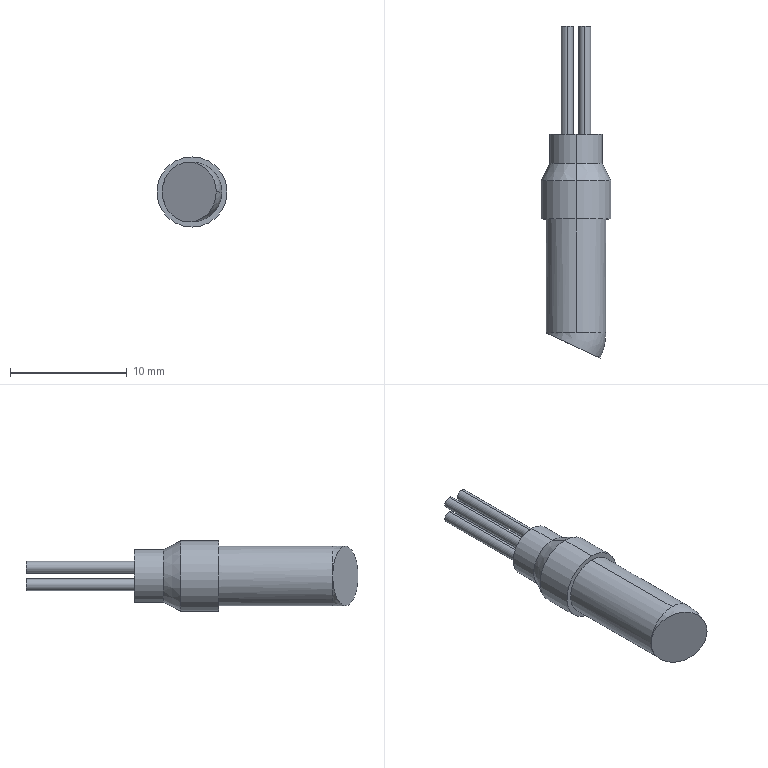Part | SolidWorks | features BaseBody 1 | 1 solid | 25 faces | box 6 x 28.381 x 6 mm | volume 414.888 mm3 | cylinder 14 | plane 7 | spline 2 | cone 2 | commonest cylinder face diameters 1 x8 4.5 x2 5.1 x2 6 x2
STEP:
#1=CARTESIAN_POINT('',(2.55,68.684,0.));
#2=VERTEX_POINT('',#1);
#3=CARTESIAN_POINT('',(0.,68.684,-2.55));
#4=VERTEX_POINT('',#3);
#5=CARTESIAN_POINT('',(0.,68.684,0.));
#6=DIRECTION('',(0.,1.,0.));
#7=DIRECTION('',(0.,0.,1.));
#8=AXIS2_PLACEMENT_3D('',#5,#6,#7);
#9=CIRCLE('',#8,2.55);
#10=EDGE_CURVE('',#2,#4,#9,.T.);
#11=ORIENTED_EDGE('',*,*,#10,.T.);
#12=CARTESIAN_POINT('',(0.,78.399,-2.55));
#13=VERTEX_POINT('',#12);
#14=CARTESIAN_POINT('',(0.,80.649,-2.55));
#15=DIRECTION('',(0.,1.,0.));
#16=VECTOR('',#15,1000.);
#17=LINE('',#14,#16);
#18=EDGE_CURVE('',#4,#13,#17,.T.);
#19=ORIENTED_EDGE('',*,*,#18,.T.);
#20=CARTESIAN_POINT('',(0.,78.399,2.55));
#21=VERTEX_POINT('',#20);
#22=CARTESIAN_POINT('',(0.,78.399,0.));
#23=DIRECTION('',(0.,-1.,0.));
#24=DIRECTION('',(0.,0.,1.));
#25=AXIS2_PLACEMENT_3D('',#22,#23,#24);
#26=CIRCLE('',#25,2.55);
#27=EDGE_CURVE('',#13,#21,#26,.T.);
#28=ORIENTED_EDGE('',*,*,#27,.T.);
#29=CARTESIAN_POINT('',(0.,68.684,2.55));
#30=VERTEX_POINT('',#29);
#31=CARTESIAN_POINT('',(0.,80.649,2.55));
#32=DIRECTION('',(0.,1.,0.));
#33=VECTOR('',#32,1000.);
#34=LINE('',#31,#33);
#35=EDGE_CURVE('',#30,#21,#34,.T.);
#36=ORIENTED_EDGE('',*,*,#35,.F.);
#37=CARTESIAN_POINT('',(0.,68.684,0.));
#38=DIRECTION('',(0.,1.,0.));
#39=DIRECTION('',(0.,0.,1.));
#40=AXIS2_PLACEMENT_3D('',#37,#38,#39);
#41=CIRCLE('',#40,2.55);
#42=EDGE_CURVE('',#30,#2,#41,.T.);
#43=ORIENTED_EDGE('',*,*,#42,.T.);
#44=EDGE_LOOP('',(#11,#19,#28,#36,#43));
#45=FACE_OUTER_BOUND('',#44,.T.);
#46=CARTESIAN_POINT('',(0.,80.649,0.));
#47=DIRECTION('',(0.,1.,0.));
#48=DIRECTION('',(0.,0.,1.));
#49=AXIS2_PLACEMENT_3D('',#46,#47,#48);
#50=CYLINDRICAL_SURFACE('',#49,2.55);
#51=ADVANCED_FACE('',(#45),#50,.T.);
#52=CARTESIAN_POINT('',(2.069,66.514,0.));
#53=VERTEX_POINT('',#52);
#54=CARTESIAN_POINT('',(-2.553,68.67,0.));
#55=VERTEX_POINT('',#54);
#56=CARTESIAN_POINT('',(2.069,66.514,0.));
#57=CARTESIAN_POINT('',(2.069,66.514,-0.1685));
#58=CARTESIAN_POINT('',(2.054,66.521,-0.3342));
#59=CARTESIAN_POINT('',(1.995,66.549,-0.6601));
#60=CARTESIAN_POINT('',(1.951,66.569,-0.822));
#61=CARTESIAN_POINT('',(1.835,66.623,-1.131));
#62=CARTESIAN_POINT('',(1.764,66.657,-1.277));
#63=CARTESIAN_POINT('',(1.596,66.735,-1.555));
#64=CARTESIAN_POINT('',(1.498,66.78,-1.686));
#65=CARTESIAN_POINT('',(1.285,66.88,-1.921));
#66=CARTESIAN_POINT('',(1.169,66.934,-2.027));
#67=CARTESIAN_POINT('',(0.916,67.052,-2.213));
#68=CARTESIAN_POINT('',(0.7815,67.115,-2.292));
#69=CARTESIAN_POINT('',(0.5033,67.244,-2.419));
#70=CARTESIAN_POINT('',(0.3577,67.312,-2.468));
#71=CARTESIAN_POINT('',(0.05933,67.451,-2.534));
#72=CARTESIAN_POINT('',(-0.09064,67.521,-2.55));
#73=CARTESIAN_POINT('',(-0.3921,67.662,-2.55));
#74=CARTESIAN_POINT('',(-0.5452,67.733,-2.533));
#75=CARTESIAN_POINT('',(-0.8416,67.871,-2.468));
#76=CARTESIAN_POINT('',(-0.9857,67.939,-2.42));
#77=CARTESIAN_POINT('',(-1.266,68.069,-2.292));
#78=CARTESIAN_POINT('',(-1.401,68.132,-2.213));
#79=CARTESIAN_POINT('',(-1.651,68.249,-2.028));
#80=CARTESIAN_POINT('',(-1.768,68.303,-1.923));
#81=CARTESIAN_POINT('',(-1.984,68.404,-1.685));
#82=CARTESIAN_POINT('',(-2.08,68.449,-1.555));
#83=CARTESIAN_POINT('',(-2.247,68.527,-1.279));
#84=CARTESIAN_POINT('',(-2.319,68.561,-1.13));
#85=CARTESIAN_POINT('',(-2.435,68.615,-0.8212));
#86=CARTESIAN_POINT('',(-2.479,68.635,-0.6622));
#87=CARTESIAN_POINT('',(-2.538,68.663,-0.3354));
#88=CARTESIAN_POINT('',(-2.553,68.67,-0.1664));
#89=CARTESIAN_POINT('',(-2.553,68.67,0.));
#90=B_SPLINE_CURVE_WITH_KNOTS('',3,(#56,#57,#58,#59,#60,#61,#62,#63,#64,#65,#66,#67,#68,#69,#70,#71,#72,#73,#74,#75,#76,#77,#78,#79,#80,#81,#82,#83,#84,#85,#86,#87,#88,#89),.UNSPECIFIED.,.F.,.F.,(4,2,2,2,2,2,2,2,2,2,2,2,2,2,2,2,4),(0.,0.0004983,0.0009966,0.001495,0.001993,0.002491,0.00299,0.003488,0.003986,0.004485,0.004983,0.005481,0.005979,0.006478,0.006976,0.007474,0.007972),.UNSPECIFIED.);
#91=EDGE_CURVE('',#53,#55,#90,.T.);
#92=ORIENTED_EDGE('',*,*,#91,.T.);
#93=CARTESIAN_POINT('',(-2.55,68.684,0.));
#94=VERTEX_POINT('',#93);
#95=CARTESIAN_POINT('',(-2.585,68.684,0.));
#96=DIRECTION('',(0.,0.,1.));
#97=DIRECTION('',(1.,0.,0.));
#98=AXIS2_PLACEMENT_3D('',#95,#96,#97);
#99=CIRCLE('',#98,0.035);
#100=EDGE_CURVE('',#55,#94,#99,.T.);
#101=ORIENTED_EDGE('',*,*,#100,.T.);
#102=CARTESIAN_POINT('',(0.,68.684,0.));
#103=DIRECTION('',(0.,1.,0.));
#104=DIRECTION('',(0.,0.,1.));
#105=AXIS2_PLACEMENT_3D('',#102,#103,#104);
#106=CIRCLE('',#105,2.55);
#107=EDGE_CURVE('',#4,#94,#106,.T.);
#108=ORIENTED_EDGE('',*,*,#107,.F.);
#109=ORIENTED_EDGE('',*,*,#10,.F.);
#110=CARTESIAN_POINT('',(-2.585,68.684,0.));
#111=DIRECTION('',(0.,0.,1.));
#112=DIRECTION('',(1.,0.,0.));
#113=AXIS2_PLACEMENT_3D('',#110,#111,#112);
#114=CIRCLE('',#113,5.135);
#115=EDGE_CURVE('',#53,#2,#114,.T.);
#116=ORIENTED_EDGE('',*,*,#115,.F.);
#117=EDGE_LOOP('',(#92,#101,#108,#109,#116));
#118=FACE_OUTER_BOUND('',#117,.T.);
#119=CARTESIAN_POINT('',(2.069,66.514,0.));
#120=CARTESIAN_POINT('',(2.387,67.197,0.));
#121=CARTESIAN_POINT('',(2.55,67.932,0.));
#122=CARTESIAN_POINT('',(2.55,68.684,0.));
#123=CARTESIAN_POINT('',(2.069,66.514,-5.1));
#124=CARTESIAN_POINT('',(2.387,67.197,-5.1));
#125=CARTESIAN_POINT('',(2.55,67.932,-5.1));
#126=CARTESIAN_POINT('',(2.55,68.684,-5.1));
#127=CARTESIAN_POINT('',(-2.553,68.67,-5.1));
#128=CARTESIAN_POINT('',(-2.551,68.674,-5.1));
#129=CARTESIAN_POINT('',(-2.55,68.679,-5.1));
#130=CARTESIAN_POINT('',(-2.55,68.684,-5.1));
#131=CARTESIAN_POINT('',(-2.553,68.67,0.));
#132=CARTESIAN_POINT('',(-2.551,68.674,0.));
#133=CARTESIAN_POINT('',(-2.55,68.679,0.));
#134=CARTESIAN_POINT('',(-2.55,68.684,0.));
#135=(BOUNDED_SURFACE()B_SPLINE_SURFACE(3,3,((#119,#120,#121,#122),(#123,#124,#125,#126),(#127,#128,#129,#130),(#131,#132,#133,#134)),.UNSPECIFIED.,.F.,.F.,.F.)B_SPLINE_SURFACE_WITH_KNOTS((4,4),(4,4),(0.,1.),(0.,1.),.UNSPECIFIED.)GEOMETRIC_REPRESENTATION_ITEM()RATIONAL_B_SPLINE_SURFACE(((1.,0.9842,0.9842,1.),(0.3333,0.3281,0.3281,0.3333),(0.3333,0.3281,0.3281,0.3333),(1.,0.9842,0.9842,1.)))REPRESENTATION_ITEM('')SURFACE());
#136=ADVANCED_FACE('',(#118),#135,.T.);
#137=CARTESIAN_POINT('',(0.,78.399,3.));
#138=VERTEX_POINT('',#137);
#139=CARTESIAN_POINT('',(0.,78.399,-3.));
#140=VERTEX_POINT('',#139);
#141=CARTESIAN_POINT('',(0.,78.399,0.));
#142=DIRECTION('',(0.,1.,0.));
#143=DIRECTION('',(0.,0.,1.));
#144=AXIS2_PLACEMENT_3D('',#141,#142,#143);
#145=CIRCLE('',#144,3.);
#146=EDGE_CURVE('',#138,#140,#145,.T.);
#147=ORIENTED_EDGE('',*,*,#146,.T.);
#148=CARTESIAN_POINT('',(0.,81.649,-3.));
#149=VERTEX_POINT('',#148);
#150=CARTESIAN_POINT('',(0.,78.399,-3.));
#151=DIRECTION('',(0.,1.,0.));
#152=VECTOR('',#151,1000.);
#153=LINE('',#150,#152);
#154=EDGE_CURVE('',#140,#149,#153,.T.);
#155=ORIENTED_EDGE('',*,*,#154,.T.);
#156=CARTESIAN_POINT('',(0.,81.649,3.));
#157=VERTEX_POINT('',#156);
#158=CARTESIAN_POINT('',(0.,81.649,0.));
#159=DIRECTION('',(0.,-1.,0.));
#160=DIRECTION('',(0.,0.,1.));
#161=AXIS2_PLACEMENT_3D('',#158,#159,#160);
#162=CIRCLE('',#161,3.);
#163=EDGE_CURVE('',#149,#157,#162,.T.);
#164=ORIENTED_EDGE('',*,*,#163,.T.);
#165=CARTESIAN_POINT('',(0.,78.399,3.));
#166=DIRECTION('',(0.,1.,0.));
#167=VECTOR('',#166,1000.);
#168=LINE('',#165,#167);
#169=EDGE_CURVE('',#138,#157,#168,.T.);
#170=ORIENTED_EDGE('',*,*,#169,.F.);
#171=EDGE_LOOP('',(#147,#155,#164,#170));
#172=FACE_OUTER_BOUND('',#171,.T.);
#173=CARTESIAN_POINT('',(0.,78.399,0.));
#174=DIRECTION('',(0.,1.,0.));
#175=DIRECTION('',(0.,0.,1.));
#176=AXIS2_PLACEMENT_3D('',#173,#174,#175);
#177=CYLINDRICAL_SURFACE('',#176,3.);
#178=ADVANCED_FACE('',(#172),#177,.T.);
#179=CARTESIAN_POINT('',(0.,83.149,-2.25));
#180=VERTEX_POINT('',#179);
#181=CARTESIAN_POINT('',(0.,83.149,2.25));
#182=VERTEX_POINT('',#181);
#183=CARTESIAN_POINT('',(0.,83.149,0.));
#184=DIRECTION('',(0.,-1.,0.));
#185=DIRECTION('',(0.,0.,-1.));
#186=AXIS2_PLACEMENT_3D('',#183,#184,#185);
#187=CIRCLE('',#186,2.25);
#188=EDGE_CURVE('',#180,#182,#187,.T.);
#189=ORIENTED_EDGE('',*,*,#188,.T.);
#190=CARTESIAN_POINT('',(0.,81.649,3.));
#191=DIRECTION('',(0.,-0.8944,0.4472));
#192=VECTOR('',#191,1000.);
#193=LINE('',#190,#192);
#194=EDGE_CURVE('',#182,#157,#193,.T.);
#195=ORIENTED_EDGE('',*,*,#194,.T.);
#196=ORIENTED_EDGE('',*,*,#163,.F.);
#197=CARTESIAN_POINT('',(0.,81.649,-3.));
#198=DIRECTION('',(0.,-0.8944,-0.4472));
#199=VECTOR('',#198,1000.);
#200=LINE('',#197,#199);
#201=EDGE_CURVE('',#180,#149,#200,.T.);
#202=ORIENTED_EDGE('',*,*,#201,.F.);
#203=EDGE_LOOP('',(#189,#195,#196,#202));
#204=FACE_OUTER_BOUND('',#203,.T.);
#205=CARTESIAN_POINT('',(0.,81.649,0.));
#206=DIRECTION('',(0.,-1.,0.));
#207=DIRECTION('',(0.,0.,-1.));
#208=AXIS2_PLACEMENT_3D('',#205,#206,#207);
#209=CONICAL_SURFACE('',#208,3.,0.4636);
#210=ADVANCED_FACE('',(#204),#209,.T.);
#211=ORIENTED_EDGE('',*,*,#188,.F.);
#212=CARTESIAN_POINT('',(0.,85.649,-2.25));
#213=VERTEX_POINT('',#212);
#214=CARTESIAN_POINT('',(0.,78.399,-2.25));
#215=DIRECTION('',(0.,1.,0.));
#216=VECTOR('',#215,1000.);
#217=LINE('',#214,#216);
#218=EDGE_CURVE('',#180,#213,#217,.T.);
#219=ORIENTED_EDGE('',*,*,#218,.T.);
#220=CARTESIAN_POINT('',(0.,85.649,2.25));
#221=VERTEX_POINT('',#220);
#222=CARTESIAN_POINT('',(0.,85.649,0.));
#223=DIRECTION('',(0.,-1.,0.));
#224=DIRECTION('',(0.,0.,1.));
#225=AXIS2_PLACEMENT_3D('',#222,#223,#224);
#226=CIRCLE('',#225,2.25);
#227=EDGE_CURVE('',#213,#221,#226,.T.);
#228=ORIENTED_EDGE('',*,*,#227,.T.);
#229=CARTESIAN_POINT('',(0.,78.399,2.25));
#230=DIRECTION('',(0.,1.,0.));
#231=VECTOR('',#230,1000.);
#232=LINE('',#229,#231);
#233=EDGE_CURVE('',#182,#221,#232,.T.);
#234=ORIENTED_EDGE('',*,*,#233,.F.);
#235=EDGE_LOOP('',(#211,#219,#228,#234));
#236=FACE_OUTER_BOUND('',#235,.T.);
#237=CARTESIAN_POINT('',(0.,78.399,0.));
#238=DIRECTION('',(0.,1.,0.));
#239=DIRECTION('',(0.,0.,1.));
#240=AXIS2_PLACEMENT_3D('',#237,#238,#239);
#241=CYLINDRICAL_SURFACE('',#240,2.25);
#242=ADVANCED_FACE('',(#236),#241,.T.);
#243=CARTESIAN_POINT('',(0.75,85.649,-0.25));
#244=VERTEX_POINT('',#243);
#245=CARTESIAN_POINT('',(0.75,85.649,-1.25));
#246=VERTEX_POINT('',#245);
#247=CARTESIAN_POINT('',(0.75,85.649,-0.75));
#248=DIRECTION('',(0.,1.,0.));
#249=DIRECTION('',(0.,0.,1.));
#250=AXIS2_PLACEMENT_3D('',#247,#248,#249);
#251=CIRCLE('',#250,0.5);
#252=EDGE_CURVE('',#244,#246,#251,.T.);
#253=ORIENTED_EDGE('',*,*,#252,.T.);
#254=CARTESIAN_POINT('',(0.75,94.895,-1.25));
#255=VERTEX_POINT('',#254);
#256=CARTESIAN_POINT('',(0.75,94.895,-1.25));
#257=DIRECTION('',(0.,1.,0.));
#258=VECTOR('',#257,1000.);
#259=LINE('',#256,#258);
#260=EDGE_CURVE('',#246,#255,#259,.T.);
#261=ORIENTED_EDGE('',*,*,#260,.T.);
#262=CARTESIAN_POINT('',(0.75,94.895,-0.25));
#263=VERTEX_POINT('',#262);
#264=CARTESIAN_POINT('',(0.75,94.895,-0.75));
#265=DIRECTION('',(0.,-1.,0.));
#266=DIRECTION('',(0.,0.,1.));
#267=AXIS2_PLACEMENT_3D('',#264,#265,#266);
#268=CIRCLE('',#267,0.5);
#269=EDGE_CURVE('',#255,#263,#268,.T.);
#270=ORIENTED_EDGE('',*,*,#269,.T.);
#271=CARTESIAN_POINT('',(0.75,94.895,-0.25));
#272=DIRECTION('',(0.,1.,0.));
#273=VECTOR('',#272,1000.);
#274=LINE('',#271,#273);
#275=EDGE_CURVE('',#244,#263,#274,.T.);
#276=ORIENTED_EDGE('',*,*,#275,.F.);
#277=EDGE_LOOP('',(#253,#261,#270,#276));
#278=FACE_OUTER_BOUND('',#277,.T.);
#279=CARTESIAN_POINT('',(0.75,94.895,-0.75));
#280=DIRECTION('',(0.,1.,0.));
#281=DIRECTION('',(0.,0.,1.));
#282=AXIS2_PLACEMENT_3D('',#279,#280,#281);
#283=CYLINDRICAL_SURFACE('',#282,0.5);
#284=ADVANCED_FACE('',(#278),#283,.T.);
#285=CARTESIAN_POINT('',(-0.75,85.649,-0.25));
#286=VERTEX_POINT('',#285);
#287=CARTESIAN_POINT('',(-0.75,85.649,-1.25));
#288=VERTEX_POINT('',#287);
#289=CARTESIAN_POINT('',(-0.75,85.649,-0.75));
#290=DIRECTION('',(0.,1.,0.));
#291=DIRECTION('',(0.,0.,1.));
#292=AXIS2_PLACEMENT_3D('',#289,#290,#291);
#293=CIRCLE('',#292,0.5);
#294=EDGE_CURVE('',#286,#288,#293,.T.);
#295=ORIENTED_EDGE('',*,*,#294,.T.);
#296=CARTESIAN_POINT('',(-0.75,94.895,-1.25));
#297=VERTEX_POINT('',#296);
#298=CARTESIAN_POINT('',(-0.75,94.895,-1.25));
#299=DIRECTION('',(0.,1.,0.));
#300=VECTOR('',#299,1000.);
#301=LINE('',#298,#300);
#302=EDGE_CURVE('',#288,#297,#301,.T.);
#303=ORIENTED_EDGE('',*,*,#302,.T.);
#304=CARTESIAN_POINT('',(-0.75,94.895,-0.25));
#305=VERTEX_POINT('',#304);
#306=CARTESIAN_POINT('',(-0.75,94.895,-0.75));
#307=DIRECTION('',(0.,-1.,0.));
#308=DIRECTION('',(0.,0.,1.));
#309=AXIS2_PLACEMENT_3D('',#306,#307,#308);
#310=CIRCLE('',#309,0.5);
#311=EDGE_CURVE('',#297,#305,#310,.T.);
#312=ORIENTED_EDGE('',*,*,#311,.T.);
#313=CARTESIAN_POINT('',(-0.75,94.895,-0.25));
#314=DIRECTION('',(0.,1.,0.));
#315=VECTOR('',#314,1000.);
#316=LINE('',#313,#315);
#317=EDGE_CURVE('',#286,#305,#316,.T.);
#318=ORIENTED_EDGE('',*,*,#317,.F.);
#319=EDGE_LOOP('',(#295,#303,#312,#318));
#320=FACE_OUTER_BOUND('',#319,.T.);
#321=CARTESIAN_POINT('',(-0.75,94.895,-0.75));
#322=DIRECTION('',(0.,1.,0.));
#323=DIRECTION('',(0.,0.,1.));
#324=AXIS2_PLACEMENT_3D('',#321,#322,#323);
#325=CYLINDRICAL_SURFACE('',#324,0.5);
#326=ADVANCED_FACE('',(#320),#325,.T.);
#327=CARTESIAN_POINT('',(-0.75,85.649,1.25));
#328=VERTEX_POINT('',#327);
#329=CARTESIAN_POINT('',(-0.75,85.649,0.25));
#330=VERTEX_POINT('',#329);
#331=CARTESIAN_POINT('',(-0.75,85.649,0.75));
#332=DIRECTION('',(0.,1.,0.));
#333=DIRECTION('',(0.,0.,1.));
#334=AXIS2_PLACEMENT_3D('',#331,#332,#333);
#335=CIRCLE('',#334,0.5);
#336=EDGE_CURVE('',#328,#330,#335,.T.);
#337=ORIENTED_EDGE('',*,*,#336,.T.);
#338=CARTESIAN_POINT('',(-0.75,94.895,0.25));
#339=VERTEX_POINT('',#338);
#340=CARTESIAN_POINT('',(-0.75,94.895,0.25));
#341=DIRECTION('',(0.,1.,0.));
#342=VECTOR('',#341,1000.);
#343=LINE('',#340,#342);
#344=EDGE_CURVE('',#330,#339,#343,.T.);
#345=ORIENTED_EDGE('',*,*,#344,.T.);
#346=CARTESIAN_POINT('',(-0.75,94.895,1.25));
#347=VERTEX_POINT('',#346);
#348=CARTESIAN_POINT('',(-0.75,94.895,0.75));
#349=DIRECTION('',(0.,-1.,0.));
#350=DIRECTION('',(0.,0.,1.));
#351=AXIS2_PLACEMENT_3D('',#348,#349,#350);
#352=CIRCLE('',#351,0.5);
#353=EDGE_CURVE('',#339,#347,#352,.T.);
#354=ORIENTED_EDGE('',*,*,#353,.T.);
#355=CARTESIAN_POINT('',(-0.75,94.895,1.25));
#356=DIRECTION('',(0.,1.,0.));
#357=VECTOR('',#356,1000.);
#358=LINE('',#355,#357);
#359=EDGE_CURVE('',#328,#347,#358,.T.);
#360=ORIENTED_EDGE('',*,*,#359,.F.);
#361=EDGE_LOOP('',(#337,#345,#354,#360));
#362=FACE_OUTER_BOUND('',#361,.T.);
#363=CARTESIAN_POINT('',(-0.75,94.895,0.75));
#364=DIRECTION('',(0.,1.,0.));
#365=DIRECTION('',(0.,0.,1.));
#366=AXIS2_PLACEMENT_3D('',#363,#364,#365);
#367=CYLINDRICAL_SURFACE('',#366,0.5);
#368=ADVANCED_FACE('',(#362),#367,.T.);
#369=CARTESIAN_POINT('',(0.75,85.649,1.25));
#370=VERTEX_POINT('',#369);
#371=CARTESIAN_POINT('',(0.75,85.649,0.25));
#372=VERTEX_POINT('',#371);
#373=CARTESIAN_POINT('',(0.75,85.649,0.75));
#374=DIRECTION('',(0.,1.,0.));
#375=DIRECTION('',(0.,0.,1.));
#376=AXIS2_PLACEMENT_3D('',#373,#374,#375);
#377=CIRCLE('',#376,0.5);
#378=EDGE_CURVE('',#370,#372,#377,.T.);
#379=ORIENTED_EDGE('',*,*,#378,.T.);
#380=CARTESIAN_POINT('',(0.75,94.895,0.25));
#381=VERTEX_POINT('',#380);
#382=CARTESIAN_POINT('',(0.75,94.895,0.25));
#383=DIRECTION('',(0.,1.,0.));
#384=VECTOR('',#383,1000.);
#385=LINE('',#382,#384);
#386=EDGE_CURVE('',#372,#381,#385,.T.);
#387=ORIENTED_EDGE('',*,*,#386,.T.);
#388=CARTESIAN_POINT('',(0.75,94.895,1.25));
#389=VERTEX_POINT('',#388);
#390=CARTESIAN_POINT('',(0.75,94.895,0.75));
#391=DIRECTION('',(0.,-1.,0.));
#392=DIRECTION('',(0.,0.,1.));
#393=AXIS2_PLACEMENT_3D('',#390,#391,#392);
#394=CIRCLE('',#393,0.5);
#395=EDGE_CURVE('',#381,#389,#394,.T.);
#396=ORIENTED_EDGE('',*,*,#395,.T.);
#397=CARTESIAN_POINT('',(0.75,94.895,1.25));
#398=DIRECTION('',(0.,1.,0.));
#399=VECTOR('',#398,1000.);
#400=LINE('',#397,#399);
#401=EDGE_CURVE('',#370,#389,#400,.T.);
#402=ORIENTED_EDGE('',*,*,#401,.F.);
#403=EDGE_LOOP('',(#379,#387,#396,#402));
#404=FACE_OUTER_BOUND('',#403,.T.);
#405=CARTESIAN_POINT('',(0.75,94.895,0.75));
#406=DIRECTION('',(0.,1.,0.));
#407=DIRECTION('',(0.,0.,1.));
#408=AXIS2_PLACEMENT_3D('',#405,#406,#407);
#409=CYLINDRICAL_SURFACE('',#408,0.5);
#410=ADVANCED_FACE('',(#404),#409,.T.);
#411=ORIENTED_EDGE('',*,*,#18,.F.);
#412=ORIENTED_EDGE('',*,*,#107,.T.);
#413=CARTESIAN_POINT('',(0.,68.684,0.));
#414=DIRECTION('',(0.,1.,0.));
#415=DIRECTION('',(0.,0.,1.));
#416=AXIS2_PLACEMENT_3D('',#413,#414,#415);
#417=CIRCLE('',#416,2.55);
#418=EDGE_CURVE('',#94,#30,#417,.T.);
#419=ORIENTED_EDGE('',*,*,#418,.T.);
#420=ORIENTED_EDGE('',*,*,#35,.T.);
#421=CARTESIAN_POINT('',(0.,78.399,0.));
#422=DIRECTION('',(0.,-1.,0.));
#423=DIRECTION('',(0.,0.,1.));
#424=AXIS2_PLACEMENT_3D('',#421,#422,#423);
#425=CIRCLE('',#424,2.55);
#426=EDGE_CURVE('',#21,#13,#425,.T.);
#427=ORIENTED_EDGE('',*,*,#426,.T.);
#428=EDGE_LOOP('',(#411,#412,#419,#420,#427));
#429=FACE_OUTER_BOUND('',#428,.T.);
#430=CARTESIAN_POINT('',(0.,80.649,0.));
#431=DIRECTION('',(0.,1.,0.));
#432=DIRECTION('',(0.,0.,1.));
#433=AXIS2_PLACEMENT_3D('',#430,#431,#432);
#434=CYLINDRICAL_SURFACE('',#433,2.55);
#435=ADVANCED_FACE('',(#429),#434,.T.);
#436=ORIENTED_EDGE('',*,*,#146,.F.);
#437=CARTESIAN_POINT('',(0.,78.399,0.));
#438=DIRECTION('',(0.,1.,0.));
#439=DIRECTION('',(0.,0.,1.));
#440=AXIS2_PLACEMENT_3D('',#437,#438,#439);
#441=CIRCLE('',#440,3.);
#442=EDGE_CURVE('',#140,#138,#441,.T.);
#443=ORIENTED_EDGE('',*,*,#442,.F.);
#444=EDGE_LOOP('',(#436,#443));
#445=FACE_OUTER_BOUND('',#444,.T.);
#446=ORIENTED_EDGE('',*,*,#426,.F.);
#447=ORIENTED_EDGE('',*,*,#27,.F.);
#448=EDGE_LOOP('',(#446,#447));
#449=FACE_BOUND('',#448,.T.);
#450=CARTESIAN_POINT('',(3.,78.399,0.));
#451=DIRECTION('',(0.,1.,0.));
#452=DIRECTION('',(0.,0.,1.));
#453=AXIS2_PLACEMENT_3D('',#450,#451,#452);
#454=PLANE('',#453);
#455=ADVANCED_FACE('',(#445,#449),#454,.F.);
#456=ORIENTED_EDGE('',*,*,#100,.F.);
#457=CARTESIAN_POINT('',(-2.553,68.67,0.));
#458=CARTESIAN_POINT('',(-2.553,68.67,0.1664));
#459=CARTESIAN_POINT('',(-2.539,68.663,0.3318));
#460=CARTESIAN_POINT('',(-2.48,68.635,0.6604));
#461=CARTESIAN_POINT('',(-2.435,68.615,0.8216));
#462=CARTESIAN_POINT('',(-2.263,68.534,1.282));
#463=CARTESIAN_POINT('',(-2.09,68.454,1.567));
#464=CARTESIAN_POINT('',(-1.771,68.305,1.919));
#465=CARTESIAN_POINT('',(-1.652,68.249,2.027));
#466=CARTESIAN_POINT('',(-1.401,68.132,2.213));
#467=CARTESIAN_POINT('',(-1.268,68.07,2.291));
#468=CARTESIAN_POINT('',(-0.9889,67.94,2.419));
#469=CARTESIAN_POINT('',(-0.8419,67.872,2.468));
#470=CARTESIAN_POINT('',(-0.5465,67.734,2.533));
#471=CARTESIAN_POINT('',(-0.3965,67.664,2.55));
#472=CARTESIAN_POINT('',(-0.09177,67.522,2.55));
#473=CARTESIAN_POINT('',(0.05903,67.451,2.534));
#474=CARTESIAN_POINT('',(0.3543,67.314,2.469));
#475=CARTESIAN_POINT('',(0.5008,67.245,2.42));
#476=CARTESIAN_POINT('',(0.7811,67.115,2.293));
#477=CARTESIAN_POINT('',(0.9139,67.053,2.214));
#478=CARTESIAN_POINT('',(1.165,66.936,2.03));
#479=CARTESIAN_POINT('',(1.284,66.88,1.922));
#480=CARTESIAN_POINT('',(1.498,66.781,1.687));
#481=CARTESIAN_POINT('',(1.593,66.736,1.559));
#482=CARTESIAN_POINT('',(1.762,66.657,1.28));
#483=CARTESIAN_POINT('',(1.834,66.624,1.132));
#484=CARTESIAN_POINT('',(2.008,66.543,0.6716));
#485=CARTESIAN_POINT('',(2.069,66.514,0.3369));
#486=CARTESIAN_POINT('',(2.069,66.514,0.));
#487=B_SPLINE_CURVE_WITH_KNOTS('',3,(#457,#458,#459,#460,#461,#462,#463,#464,#465,#466,#467,#468,#469,#470,#471,#472,#473,#474,#475,#476,#477,#478,#479,#480,#481,#482,#483,#484,#485,#486),.UNSPECIFIED.,.F.,.F.,(4,2,2,2,2,2,2,2,2,2,2,2,2,2,4),(0.007972,0.008471,0.008969,0.009965,0.01046,0.01096,0.01146,0.01196,0.01246,0.01295,0.01345,0.01395,0.01445,0.01495,0.01594),.UNSPECIFIED.);
#488=EDGE_CURVE('',#55,#53,#487,.T.);
#489=ORIENTED_EDGE('',*,*,#488,.T.);
#490=ORIENTED_EDGE('',*,*,#115,.T.);
#491=ORIENTED_EDGE('',*,*,#42,.F.);
#492=ORIENTED_EDGE('',*,*,#418,.F.);
#493=EDGE_LOOP('',(#456,#489,#490,#491,#492));
#494=FACE_OUTER_BOUND('',#493,.T.);
#495=CARTESIAN_POINT('',(-2.553,68.67,0.));
#496=CARTESIAN_POINT('',(-2.551,68.674,0.));
#497=CARTESIAN_POINT('',(-2.55,68.679,0.));
#498=CARTESIAN_POINT('',(-2.55,68.684,0.));
#499=CARTESIAN_POINT('',(-2.553,68.67,5.1));
#500=CARTESIAN_POINT('',(-2.551,68.674,5.1));
#501=CARTESIAN_POINT('',(-2.55,68.679,5.1));
#502=CARTESIAN_POINT('',(-2.55,68.684,5.1));
#503=CARTESIAN_POINT('',(2.069,66.514,5.1));
#504=CARTESIAN_POINT('',(2.387,67.197,5.1));
#505=CARTESIAN_POINT('',(2.55,67.932,5.1));
#506=CARTESIAN_POINT('',(2.55,68.684,5.1));
#507=CARTESIAN_POINT('',(2.069,66.514,0.));
#508=CARTESIAN_POINT('',(2.387,67.197,0.));
#509=CARTESIAN_POINT('',(2.55,67.932,0.));
#510=CARTESIAN_POINT('',(2.55,68.684,0.));
#511=(BOUNDED_SURFACE()B_SPLINE_SURFACE(3,3,((#495,#496,#497,#498),(#499,#500,#501,#502),(#503,#504,#505,#506),(#507,#508,#509,#510)),.UNSPECIFIED.,.F.,.F.,.F.)B_SPLINE_SURFACE_WITH_KNOTS((4,4),(4,4),(0.,1.),(0.,1.),.UNSPECIFIED.)GEOMETRIC_REPRESENTATION_ITEM()RATIONAL_B_SPLINE_SURFACE(((1.,0.9842,0.9842,1.),(0.3333,0.3281,0.3281,0.3333),(0.3333,0.3281,0.3281,0.3333),(1.,0.9842,0.9842,1.)))REPRESENTATION_ITEM('')SURFACE());
#512=ADVANCED_FACE('',(#494),#511,.T.);
#513=ORIENTED_EDGE('',*,*,#154,.F.);
#514=ORIENTED_EDGE('',*,*,#442,.T.);
#515=ORIENTED_EDGE('',*,*,#169,.T.);
#516=CARTESIAN_POINT('',(0.,81.649,0.));
#517=DIRECTION('',(0.,-1.,0.));
#518=DIRECTION('',(0.,0.,1.));
#519=AXIS2_PLACEMENT_3D('',#516,#517,#518);
#520=CIRCLE('',#519,3.);
#521=EDGE_CURVE('',#157,#149,#520,.T.);
#522=ORIENTED_EDGE('',*,*,#521,.T.);
#523=EDGE_LOOP('',(#513,#514,#515,#522));
#524=FACE_OUTER_BOUND('',#523,.T.);
#525=CARTESIAN_POINT('',(0.,78.399,0.));
#526=DIRECTION('',(0.,1.,0.));
#527=DIRECTION('',(0.,0.,1.));
#528=AXIS2_PLACEMENT_3D('',#525,#526,#527);
#529=CYLINDRICAL_SURFACE('',#528,3.);
#530=ADVANCED_FACE('',(#524),#529,.T.);
#531=ORIENTED_EDGE('',*,*,#91,.F.);
#532=ORIENTED_EDGE('',*,*,#488,.F.);
#533=EDGE_LOOP('',(#531,#532));
#534=FACE_OUTER_BOUND('',#533,.T.);
#535=CARTESIAN_POINT('',(-0.2422,67.592,0.));
#536=DIRECTION('',(0.4226,0.9063,0.));
#537=DIRECTION('',(-0.9063,0.4226,0.));
#538=AXIS2_PLACEMENT_3D('',#535,#536,#537);
#539=PLANE('',#538);
#540=ADVANCED_FACE('',(#534),#539,.F.);
#541=ORIENTED_EDGE('',*,*,#194,.F.);
#542=CARTESIAN_POINT('',(0.,83.149,0.));
#543=DIRECTION('',(0.,-1.,0.));
#544=DIRECTION('',(0.,0.,-1.));
#545=AXIS2_PLACEMENT_3D('',#542,#543,#544);
#546=CIRCLE('',#545,2.25);
#547=EDGE_CURVE('',#182,#180,#546,.T.);
#548=ORIENTED_EDGE('',*,*,#547,.T.);
#549=ORIENTED_EDGE('',*,*,#201,.T.);
#550=ORIENTED_EDGE('',*,*,#521,.F.);
#551=EDGE_LOOP('',(#541,#548,#549,#550));
#552=FACE_OUTER_BOUND('',#551,.T.);
#553=CARTESIAN_POINT('',(0.,81.649,0.));
#554=DIRECTION('',(0.,-1.,0.));
#555=DIRECTION('',(0.,0.,-1.));
#556=AXIS2_PLACEMENT_3D('',#553,#554,#555);
#557=CONICAL_SURFACE('',#556,3.,0.4636);
#558=ADVANCED_FACE('',(#552),#557,.T.);
#559=ORIENTED_EDGE('',*,*,#218,.F.);
#560=ORIENTED_EDGE('',*,*,#547,.F.);
#561=ORIENTED_EDGE('',*,*,#233,.T.);
#562=CARTESIAN_POINT('',(0.,85.649,0.));
#563=DIRECTION('',(0.,-1.,0.));
#564=DIRECTION('',(0.,0.,1.));
#565=AXIS2_PLACEMENT_3D('',#562,#563,#564);
#566=CIRCLE('',#565,2.25);
#567=EDGE_CURVE('',#221,#213,#566,.T.);
#568=ORIENTED_EDGE('',*,*,#567,.T.);
#569=EDGE_LOOP('',(#559,#560,#561,#568));
#570=FACE_OUTER_BOUND('',#569,.T.);
#571=CARTESIAN_POINT('',(0.,78.399,0.));
#572=DIRECTION('',(0.,1.,0.));
#573=DIRECTION('',(0.,0.,1.));
#574=AXIS2_PLACEMENT_3D('',#571,#572,#573);
#575=CYLINDRICAL_SURFACE('',#574,2.25);
#576=ADVANCED_FACE('',(#570),#575,.T.);
#577=ORIENTED_EDGE('',*,*,#252,.F.);
#578=CARTESIAN_POINT('',(0.75,85.649,-0.75));
#579=DIRECTION('',(0.,1.,0.));
#580=DIRECTION('',(0.,0.,1.));
#581=AXIS2_PLACEMENT_3D('',#578,#579,#580);
#582=CIRCLE('',#581,0.5);
#583=EDGE_CURVE('',#246,#244,#582,.T.);
#584=ORIENTED_EDGE('',*,*,#583,.F.);
#585=EDGE_LOOP('',(#577,#584));
#586=FACE_BOUND('',#585,.T.);
#587=ORIENTED_EDGE('',*,*,#294,.F.);
#588=CARTESIAN_POINT('',(-0.75,85.649,-0.75));
#589=DIRECTION('',(0.,1.,0.));
#590=DIRECTION('',(0.,0.,1.));
#591=AXIS2_PLACEMENT_3D('',#588,#589,#590);
#592=CIRCLE('',#591,0.5);
#593=EDGE_CURVE('',#288,#286,#592,.T.);
#594=ORIENTED_EDGE('',*,*,#593,.F.);
#595=EDGE_LOOP('',(#587,#594));
#596=FACE_BOUND('',#595,.T.);
#597=ORIENTED_EDGE('',*,*,#336,.F.);
#598=CARTESIAN_POINT('',(-0.75,85.649,0.75));
#599=DIRECTION('',(0.,1.,0.));
#600=DIRECTION('',(0.,0.,1.));
#601=AXIS2_PLACEMENT_3D('',#598,#599,#600);
#602=CIRCLE('',#601,0.5);
#603=EDGE_CURVE('',#330,#328,#602,.T.);
#604=ORIENTED_EDGE('',*,*,#603,.F.);
#605=EDGE_LOOP('',(#597,#604));
#606=FACE_BOUND('',#605,.T.);
#607=ORIENTED_EDGE('',*,*,#378,.F.);
#608=CARTESIAN_POINT('',(0.75,85.649,0.75));
#609=DIRECTION('',(0.,1.,0.));
#610=DIRECTION('',(0.,0.,1.));
#611=AXIS2_PLACEMENT_3D('',#608,#609,#610);
#612=CIRCLE('',#611,0.5);
#613=EDGE_CURVE('',#372,#370,#612,.T.);
#614=ORIENTED_EDGE('',*,*,#613,.F.);
#615=EDGE_LOOP('',(#607,#614));
#616=FACE_BOUND('',#615,.T.);
#617=ORIENTED_EDGE('',*,*,#567,.F.);
#618=ORIENTED_EDGE('',*,*,#227,.F.);
#619=EDGE_LOOP('',(#617,#618));
#620=FACE_OUTER_BOUND('',#619,.T.);
#621=CARTESIAN_POINT('',(0.,85.649,0.));
#622=DIRECTION('',(0.,-1.,0.));
#623=DIRECTION('',(0.,0.,-1.));
#624=AXIS2_PLACEMENT_3D('',#621,#622,#623);
#625=PLANE('',#624);
#626=ADVANCED_FACE('',(#586,#596,#606,#616,#620),#625,.F.);
#627=ORIENTED_EDGE('',*,*,#260,.F.);
#628=ORIENTED_EDGE('',*,*,#583,.T.);
#629=ORIENTED_EDGE('',*,*,#275,.T.);
#630=CARTESIAN_POINT('',(0.75,94.895,-0.75));
#631=DIRECTION('',(0.,-1.,0.));
#632=DIRECTION('',(0.,0.,1.));
#633=AXIS2_PLACEMENT_3D('',#630,#631,#632);
#634=CIRCLE('',#633,0.5);
#635=EDGE_CURVE('',#263,#255,#634,.T.);
#636=ORIENTED_EDGE('',*,*,#635,.T.);
#637=EDGE_LOOP('',(#627,#628,#629,#636));
#638=FACE_OUTER_BOUND('',#637,.T.);
#639=CARTESIAN_POINT('',(0.75,94.895,-0.75));
#640=DIRECTION('',(0.,1.,0.));
#641=DIRECTION('',(0.,0.,1.));
#642=AXIS2_PLACEMENT_3D('',#639,#640,#641);
#643=CYLINDRICAL_SURFACE('',#642,0.5);
#644=ADVANCED_FACE('',(#638),#643,.T.);
#645=ORIENTED_EDGE('',*,*,#302,.F.);
#646=ORIENTED_EDGE('',*,*,#593,.T.);
#647=ORIENTED_EDGE('',*,*,#317,.T.);
#648=CARTESIAN_POINT('',(-0.75,94.895,-0.75));
#649=DIRECTION('',(0.,-1.,0.));
#650=DIRECTION('',(0.,0.,1.));
#651=AXIS2_PLACEMENT_3D('',#648,#649,#650);
#652=CIRCLE('',#651,0.5);
#653=EDGE_CURVE('',#305,#297,#652,.T.);
#654=ORIENTED_EDGE('',*,*,#653,.T.);
#655=EDGE_LOOP('',(#645,#646,#647,#654));
#656=FACE_OUTER_BOUND('',#655,.T.);
#657=CARTESIAN_POINT('',(-0.75,94.895,-0.75));
#658=DIRECTION('',(0.,1.,0.));
#659=DIRECTION('',(0.,0.,1.));
#660=AXIS2_PLACEMENT_3D('',#657,#658,#659);
#661=CYLINDRICAL_SURFACE('',#660,0.5);
#662=ADVANCED_FACE('',(#656),#661,.T.);
#663=ORIENTED_EDGE('',*,*,#344,.F.);
#664=ORIENTED_EDGE('',*,*,#603,.T.);
#665=ORIENTED_EDGE('',*,*,#359,.T.);
#666=CARTESIAN_POINT('',(-0.75,94.895,0.75));
#667=DIRECTION('',(0.,-1.,0.));
#668=DIRECTION('',(0.,0.,1.));
#669=AXIS2_PLACEMENT_3D('',#666,#667,#668);
#670=CIRCLE('',#669,0.5);
#671=EDGE_CURVE('',#347,#339,#670,.T.);
#672=ORIENTED_EDGE('',*,*,#671,.T.);
#673=EDGE_LOOP('',(#663,#664,#665,#672));
#674=FACE_OUTER_BOUND('',#673,.T.);
#675=CARTESIAN_POINT('',(-0.75,94.895,0.75));
#676=DIRECTION('',(0.,1.,0.));
#677=DIRECTION('',(0.,0.,1.));
#678=AXIS2_PLACEMENT_3D('',#675,#676,#677);
#679=CYLINDRICAL_SURFACE('',#678,0.5);
#680=ADVANCED_FACE('',(#674),#679,.T.);
#681=ORIENTED_EDGE('',*,*,#386,.F.);
#682=ORIENTED_EDGE('',*,*,#613,.T.);
#683=ORIENTED_EDGE('',*,*,#401,.T.);
#684=CARTESIAN_POINT('',(0.75,94.895,0.75));
#685=DIRECTION('',(0.,-1.,0.));
#686=DIRECTION('',(0.,0.,1.));
#687=AXIS2_PLACEMENT_3D('',#684,#685,#686);
#688=CIRCLE('',#687,0.5);
#689=EDGE_CURVE('',#389,#381,#688,.T.);
#690=ORIENTED_EDGE('',*,*,#689,.T.);
#691=EDGE_LOOP('',(#681,#682,#683,#690));
#692=FACE_OUTER_BOUND('',#691,.T.);
#693=CARTESIAN_POINT('',(0.75,94.895,0.75));
#694=DIRECTION('',(0.,1.,0.));
#695=DIRECTION('',(0.,0.,1.));
#696=AXIS2_PLACEMENT_3D('',#693,#694,#695);
#697=CYLINDRICAL_SURFACE('',#696,0.5);
#698=ADVANCED_FACE('',(#692),#697,.T.);
#699=ORIENTED_EDGE('',*,*,#635,.F.);
#700=ORIENTED_EDGE('',*,*,#269,.F.);
#701=EDGE_LOOP('',(#699,#700));
#702=FACE_OUTER_BOUND('',#701,.T.);
#703=CARTESIAN_POINT('',(0.75,94.895,-0.75));
#704=DIRECTION('',(0.,1.,0.));
#705=DIRECTION('',(0.,0.,1.));
#706=AXIS2_PLACEMENT_3D('',#703,#704,#705);
#707=PLANE('',#706);
#708=ADVANCED_FACE('',(#702),#707,.T.);
#709=ORIENTED_EDGE('',*,*,#653,.F.);
#710=ORIENTED_EDGE('',*,*,#311,.F.);
#711=EDGE_LOOP('',(#709,#710));
#712=FACE_OUTER_BOUND('',#711,.T.);
#713=CARTESIAN_POINT('',(-0.75,94.895,-0.75));
#714=DIRECTION('',(0.,1.,0.));
#715=DIRECTION('',(0.,0.,1.));
#716=AXIS2_PLACEMENT_3D('',#713,#714,#715);
#717=PLANE('',#716);
#718=ADVANCED_FACE('',(#712),#717,.T.);
#719=ORIENTED_EDGE('',*,*,#671,.F.);
#720=ORIENTED_EDGE('',*,*,#353,.F.);
#721=EDGE_LOOP('',(#719,#720));
#722=FACE_OUTER_BOUND('',#721,.T.);
#723=CARTESIAN_POINT('',(-0.75,94.895,0.75));
#724=DIRECTION('',(0.,1.,0.));
#725=DIRECTION('',(0.,0.,1.));
#726=AXIS2_PLACEMENT_3D('',#723,#724,#725);
#727=PLANE('',#726);
#728=ADVANCED_FACE('',(#722),#727,.T.);
#729=ORIENTED_EDGE('',*,*,#689,.F.);
#730=ORIENTED_EDGE('',*,*,#395,.F.);
#731=EDGE_LOOP('',(#729,#730));
#732=FACE_OUTER_BOUND('',#731,.T.);
#733=CARTESIAN_POINT('',(0.75,94.895,0.75));
#734=DIRECTION('',(0.,1.,0.));
#735=DIRECTION('',(0.,0.,1.));
#736=AXIS2_PLACEMENT_3D('',#733,#734,#735);
#737=PLANE('',#736);
#738=ADVANCED_FACE('',(#732),#737,.T.);
#739=CLOSED_SHELL('',(#51,#136,#178,#210,#242,#284,#326,#368,#410,#435,#455,#512,#530,#540,#558,#576,#626,#644,#662,#680,#698,#708,#718,#728,#738));
#740=MANIFOLD_SOLID_BREP('',#739);
#741=CARTESIAN_POINT('',(0.,0.,0.));
#742=DIRECTION('',(0.,0.,1.));
#743=DIRECTION('',(1.,0.,0.));
#744=AXIS2_PLACEMENT_3D('',#741,#742,#743);
#745=(LENGTH_UNIT()NAMED_UNIT(*)SI_UNIT(.MILLI.,.METRE.));
#746=UNCERTAINTY_MEASURE_WITH_UNIT(LENGTH_MEASURE(0.00001),#745,'','');
#747=(NAMED_UNIT(*)PLANE_ANGLE_UNIT()SI_UNIT($,.RADIAN.));
#748=(NAMED_UNIT(*)SI_UNIT($,.STERADIAN.)SOLID_ANGLE_UNIT());
#749=(GEOMETRIC_REPRESENTATION_CONTEXT(3)GLOBAL_UNCERTAINTY_ASSIGNED_CONTEXT((#746))GLOBAL_UNIT_ASSIGNED_CONTEXT((#745,#747,#748))REPRESENTATION_CONTEXT('',''));
#750=ADVANCED_BREP_SHAPE_REPRESENTATION('',(#740,#744),#749);